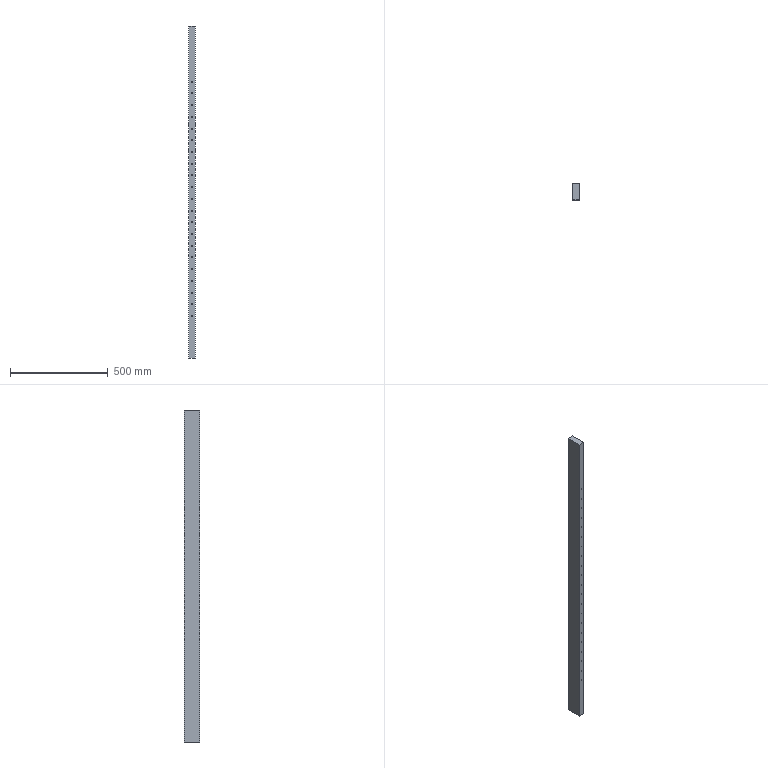Part | SolidWorks | features BaseBody 1 | 1 solid | 186 faces | box 35 x 80 x 1700 mm | volume 4708344 mm3 | cone 106 | cylinder 74 | plane 6 | commonest cylinder face diameters 5 x42 10.5 x32